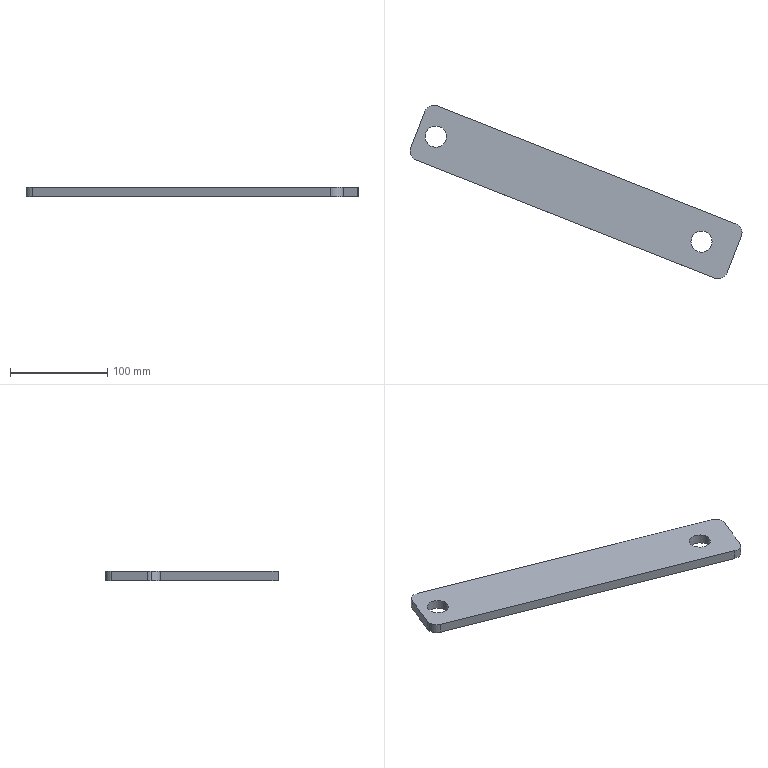Part | SolidWorks | features Extrusion 1 | 1 solid | 15 faces | box 341.614 x 178.454 x 10 mm | volume 201659 mm3 | cylinder 9 | plane 6 | commonest cylinder face diameters 20 x5 21.649 x2 22 x2
STEP:
#1=CARTESIAN_POINT('',(125.214,354.089,-1033.237));
#2=VERTEX_POINT('',#1);
#3=CARTESIAN_POINT('',(146.863,354.089,-1033.237));
#4=VERTEX_POINT('',#3);
#5=CARTESIAN_POINT('',(136.039,354.089,-1033.237));
#6=DIRECTION('',(0.,0.,1.));
#7=DIRECTION('',(1.,0.,0.));
#8=AXIS2_PLACEMENT_3D('',#5,#6,#7);
#9=CIRCLE('',#8,10.825);
#10=EDGE_CURVE('',#2,#4,#9,.T.);
#11=ORIENTED_EDGE('',*,*,#10,.T.);
#12=CARTESIAN_POINT('',(146.863,354.089,-1043.237));
#13=VERTEX_POINT('',#12);
#14=CARTESIAN_POINT('',(146.863,354.089,-1033.237));
#15=DIRECTION('',(0.,0.,-1.));
#16=VECTOR('',#15,1000.);
#17=LINE('',#14,#16);
#18=EDGE_CURVE('',#4,#13,#17,.T.);
#19=ORIENTED_EDGE('',*,*,#18,.T.);
#20=CARTESIAN_POINT('',(125.214,354.089,-1043.237));
#21=VERTEX_POINT('',#20);
#22=CARTESIAN_POINT('',(136.039,354.089,-1043.237));
#23=DIRECTION('',(0.,0.,1.));
#24=DIRECTION('',(1.,0.,0.));
#25=AXIS2_PLACEMENT_3D('',#22,#23,#24);
#26=CIRCLE('',#25,10.825);
#27=EDGE_CURVE('',#21,#13,#26,.T.);
#28=ORIENTED_EDGE('',*,*,#27,.F.);
#29=CARTESIAN_POINT('',(125.214,354.089,-1033.237));
#30=DIRECTION('',(0.,0.,-1.));
#31=VECTOR('',#30,1000.);
#32=LINE('',#29,#31);
#33=EDGE_CURVE('',#2,#21,#32,.T.);
#34=ORIENTED_EDGE('',*,*,#33,.F.);
#35=EDGE_LOOP('',(#11,#19,#28,#34));
#36=FACE_OUTER_BOUND('',#35,.T.);
#37=CARTESIAN_POINT('',(136.039,354.089,-1033.237));
#38=DIRECTION('',(0.,0.,-1.));
#39=DIRECTION('',(-1.,0.,0.));
#40=AXIS2_PLACEMENT_3D('',#37,#38,#39);
#41=CYLINDRICAL_SURFACE('',#40,10.825);
#42=ADVANCED_FACE('',(#36),#41,.F.);
#43=CARTESIAN_POINT('',(-148.238,462.051,-1033.237));
#44=VERTEX_POINT('',#43);
#45=CARTESIAN_POINT('',(-126.238,462.051,-1033.237));
#46=VERTEX_POINT('',#45);
#47=CARTESIAN_POINT('',(-137.238,462.051,-1033.237));
#48=DIRECTION('',(0.,0.,1.));
#49=DIRECTION('',(1.,0.,0.));
#50=AXIS2_PLACEMENT_3D('',#47,#48,#49);
#51=CIRCLE('',#50,11.);
#52=EDGE_CURVE('',#44,#46,#51,.T.);
#53=ORIENTED_EDGE('',*,*,#52,.T.);
#54=CARTESIAN_POINT('',(-126.238,462.051,-1043.237));
#55=VERTEX_POINT('',#54);
#56=CARTESIAN_POINT('',(-126.238,462.051,-1033.237));
#57=DIRECTION('',(0.,0.,-1.));
#58=VECTOR('',#57,1000.);
#59=LINE('',#56,#58);
#60=EDGE_CURVE('',#46,#55,#59,.T.);
#61=ORIENTED_EDGE('',*,*,#60,.T.);
#62=CARTESIAN_POINT('',(-148.238,462.051,-1043.237));
#63=VERTEX_POINT('',#62);
#64=CARTESIAN_POINT('',(-137.238,462.051,-1043.237));
#65=DIRECTION('',(0.,0.,1.));
#66=DIRECTION('',(1.,0.,0.));
#67=AXIS2_PLACEMENT_3D('',#64,#65,#66);
#68=CIRCLE('',#67,11.);
#69=EDGE_CURVE('',#63,#55,#68,.T.);
#70=ORIENTED_EDGE('',*,*,#69,.F.);
#71=CARTESIAN_POINT('',(-148.238,462.051,-1033.237));
#72=DIRECTION('',(0.,0.,-1.));
#73=VECTOR('',#72,1000.);
#74=LINE('',#71,#73);
#75=EDGE_CURVE('',#44,#63,#74,.T.);
#76=ORIENTED_EDGE('',*,*,#75,.F.);
#77=EDGE_LOOP('',(#53,#61,#70,#76));
#78=FACE_OUTER_BOUND('',#77,.T.);
#79=CARTESIAN_POINT('',(-137.238,462.051,-1033.237));
#80=DIRECTION('',(0.,0.,-1.));
#81=DIRECTION('',(-1.,0.,0.));
#82=AXIS2_PLACEMENT_3D('',#79,#80,#81);
#83=CYLINDRICAL_SURFACE('',#82,11.);
#84=ADVANCED_FACE('',(#78),#83,.F.);
#85=CARTESIAN_POINT('',(-163.887,447.124,-1033.237));
#86=VERTEX_POINT('',#85);
#87=CARTESIAN_POINT('',(-157.561,437.823,-1033.237));
#88=VERTEX_POINT('',#87);
#89=CARTESIAN_POINT('',(-153.887,447.124,-1033.237));
#90=DIRECTION('',(0.,0.,1.));
#91=DIRECTION('',(1.,0.,0.));
#92=AXIS2_PLACEMENT_3D('',#89,#90,#91);
#93=CIRCLE('',#92,10.);
#94=EDGE_CURVE('',#86,#88,#93,.T.);
#95=ORIENTED_EDGE('',*,*,#94,.F.);
#96=CARTESIAN_POINT('',(-163.887,447.124,-1043.237));
#97=VERTEX_POINT('',#96);
#98=CARTESIAN_POINT('',(-163.887,447.124,-1033.237));
#99=DIRECTION('',(0.,0.,-1.));
#100=VECTOR('',#99,1000.);
#101=LINE('',#98,#100);
#102=EDGE_CURVE('',#86,#97,#101,.T.);
#103=ORIENTED_EDGE('',*,*,#102,.T.);
#104=CARTESIAN_POINT('',(-157.561,437.823,-1043.237));
#105=VERTEX_POINT('',#104);
#106=CARTESIAN_POINT('',(-153.887,447.124,-1043.237));
#107=DIRECTION('',(0.,0.,1.));
#108=DIRECTION('',(1.,0.,0.));
#109=AXIS2_PLACEMENT_3D('',#106,#107,#108);
#110=CIRCLE('',#109,10.);
#111=EDGE_CURVE('',#97,#105,#110,.T.);
#112=ORIENTED_EDGE('',*,*,#111,.T.);
#113=CARTESIAN_POINT('',(-157.561,437.823,-1033.237));
#114=DIRECTION('',(0.,0.,-1.));
#115=VECTOR('',#114,1000.);
#116=LINE('',#113,#115);
#117=EDGE_CURVE('',#88,#105,#116,.T.);
#118=ORIENTED_EDGE('',*,*,#117,.F.);
#119=EDGE_LOOP('',(#95,#103,#112,#118));
#120=FACE_OUTER_BOUND('',#119,.T.);
#121=CARTESIAN_POINT('',(-153.887,447.124,-1033.237));
#122=DIRECTION('',(0.,0.,-1.));
#123=DIRECTION('',(-1.,0.,0.));
#124=AXIS2_PLACEMENT_3D('',#121,#122,#123);
#125=CYLINDRICAL_SURFACE('',#124,10.);
#126=ADVANCED_FACE('',(#120),#125,.T.);
#127=CARTESIAN_POINT('',(177.028,359.4,-1033.237));
#128=VERTEX_POINT('',#127);
#129=CARTESIAN_POINT('',(171.401,372.375,-1033.237));
#130=VERTEX_POINT('',#129);
#131=CARTESIAN_POINT('',(167.727,363.074,-1033.237));
#132=DIRECTION('',(0.,0.,1.));
#133=DIRECTION('',(-1.,0.,0.));
#134=AXIS2_PLACEMENT_3D('',#131,#132,#133);
#135=CIRCLE('',#134,10.);
#136=EDGE_CURVE('',#128,#130,#135,.T.);
#137=ORIENTED_EDGE('',*,*,#136,.T.);
#138=CARTESIAN_POINT('',(-135.516,493.626,-1033.237));
#139=VERTEX_POINT('',#138);
#140=CARTESIAN_POINT('',(-135.516,493.626,-1033.237));
#141=DIRECTION('',(-0.9301,0.3674,0.));
#142=VECTOR('',#141,1000.);
#143=LINE('',#140,#142);
#144=EDGE_CURVE('',#130,#139,#143,.T.);
#145=ORIENTED_EDGE('',*,*,#144,.T.);
#146=CARTESIAN_POINT('',(-148.491,488.,-1033.237));
#147=VERTEX_POINT('',#146);
#148=CARTESIAN_POINT('',(-139.19,484.326,-1033.237));
#149=DIRECTION('',(0.,0.,1.));
#150=DIRECTION('',(-1.,0.,0.));
#151=AXIS2_PLACEMENT_3D('',#148,#149,#150);
#152=CIRCLE('',#151,10.);
#153=EDGE_CURVE('',#139,#147,#152,.T.);
#154=ORIENTED_EDGE('',*,*,#153,.T.);
#155=CARTESIAN_POINT('',(-163.188,450.798,-1033.237));
#156=VERTEX_POINT('',#155);
#157=CARTESIAN_POINT('',(-148.491,488.,-1033.237));
#158=DIRECTION('',(-0.3674,-0.9301,0.));
#159=VECTOR('',#158,1000.);
#160=LINE('',#157,#159);
#161=EDGE_CURVE('',#147,#156,#160,.T.);
#162=ORIENTED_EDGE('',*,*,#161,.T.);
#163=CARTESIAN_POINT('',(-153.887,447.124,-1033.237));
#164=DIRECTION('',(0.,0.,1.));
#165=DIRECTION('',(1.,0.,0.));
#166=AXIS2_PLACEMENT_3D('',#163,#164,#165);
#167=CIRCLE('',#166,10.);
#168=EDGE_CURVE('',#156,#86,#167,.T.);
#169=ORIENTED_EDGE('',*,*,#168,.T.);
#170=ORIENTED_EDGE('',*,*,#94,.T.);
#171=CARTESIAN_POINT('',(149.356,316.572,-1033.237));
#172=VERTEX_POINT('',#171);
#173=CARTESIAN_POINT('',(-157.561,437.823,-1033.237));
#174=DIRECTION('',(0.9301,-0.3674,0.));
#175=VECTOR('',#174,1000.);
#176=LINE('',#173,#175);
#177=EDGE_CURVE('',#88,#172,#176,.T.);
#178=ORIENTED_EDGE('',*,*,#177,.T.);
#179=CARTESIAN_POINT('',(162.33,322.198,-1033.237));
#180=VERTEX_POINT('',#179);
#181=CARTESIAN_POINT('',(153.03,325.872,-1033.237));
#182=DIRECTION('',(0.,0.,1.));
#183=DIRECTION('',(-1.,0.,0.));
#184=AXIS2_PLACEMENT_3D('',#181,#182,#183);
#185=CIRCLE('',#184,10.);
#186=EDGE_CURVE('',#172,#180,#185,.T.);
#187=ORIENTED_EDGE('',*,*,#186,.T.);
#188=CARTESIAN_POINT('',(177.028,359.4,-1033.237));
#189=DIRECTION('',(0.3674,0.9301,0.));
#190=VECTOR('',#189,1000.);
#191=LINE('',#188,#190);
#192=EDGE_CURVE('',#180,#128,#191,.T.);
#193=ORIENTED_EDGE('',*,*,#192,.T.);
#194=EDGE_LOOP('',(#137,#145,#154,#162,#169,#170,#178,#187,#193));
#195=FACE_OUTER_BOUND('',#194,.T.);
#196=ORIENTED_EDGE('',*,*,#52,.F.);
#197=CARTESIAN_POINT('',(-137.238,462.051,-1033.237));
#198=DIRECTION('',(0.,0.,1.));
#199=DIRECTION('',(1.,0.,0.));
#200=AXIS2_PLACEMENT_3D('',#197,#198,#199);
#201=CIRCLE('',#200,11.);
#202=EDGE_CURVE('',#46,#44,#201,.T.);
#203=ORIENTED_EDGE('',*,*,#202,.F.);
#204=EDGE_LOOP('',(#196,#203));
#205=FACE_BOUND('',#204,.T.);
#206=ORIENTED_EDGE('',*,*,#10,.F.);
#207=CARTESIAN_POINT('',(136.039,354.089,-1033.237));
#208=DIRECTION('',(0.,0.,1.));
#209=DIRECTION('',(1.,0.,0.));
#210=AXIS2_PLACEMENT_3D('',#207,#208,#209);
#211=CIRCLE('',#210,10.825);
#212=EDGE_CURVE('',#4,#2,#211,.T.);
#213=ORIENTED_EDGE('',*,*,#212,.F.);
#214=EDGE_LOOP('',(#206,#213));
#215=FACE_BOUND('',#214,.T.);
#216=CARTESIAN_POINT('',(167.727,363.074,-1033.237));
#217=DIRECTION('',(0.,0.,-1.));
#218=DIRECTION('',(-1.,0.,0.));
#219=AXIS2_PLACEMENT_3D('',#216,#217,#218);
#220=PLANE('',#219);
#221=ADVANCED_FACE('',(#195,#205,#215),#220,.F.);
#222=ORIENTED_EDGE('',*,*,#69,.T.);
#223=CARTESIAN_POINT('',(-137.238,462.051,-1043.237));
#224=DIRECTION('',(0.,0.,1.));
#225=DIRECTION('',(1.,0.,0.));
#226=AXIS2_PLACEMENT_3D('',#223,#224,#225);
#227=CIRCLE('',#226,11.);
#228=EDGE_CURVE('',#55,#63,#227,.T.);
#229=ORIENTED_EDGE('',*,*,#228,.T.);
#230=EDGE_LOOP('',(#222,#229));
#231=FACE_BOUND('',#230,.T.);
#232=CARTESIAN_POINT('',(177.028,359.4,-1043.237));
#233=VERTEX_POINT('',#232);
#234=CARTESIAN_POINT('',(171.401,372.375,-1043.237));
#235=VERTEX_POINT('',#234);
#236=CARTESIAN_POINT('',(167.727,363.074,-1043.237));
#237=DIRECTION('',(0.,0.,1.));
#238=DIRECTION('',(-1.,0.,0.));
#239=AXIS2_PLACEMENT_3D('',#236,#237,#238);
#240=CIRCLE('',#239,10.);
#241=EDGE_CURVE('',#233,#235,#240,.T.);
#242=ORIENTED_EDGE('',*,*,#241,.F.);
#243=CARTESIAN_POINT('',(162.33,322.198,-1043.237));
#244=VERTEX_POINT('',#243);
#245=CARTESIAN_POINT('',(177.028,359.4,-1043.237));
#246=DIRECTION('',(0.3674,0.9301,0.));
#247=VECTOR('',#246,1000.);
#248=LINE('',#245,#247);
#249=EDGE_CURVE('',#244,#233,#248,.T.);
#250=ORIENTED_EDGE('',*,*,#249,.F.);
#251=CARTESIAN_POINT('',(149.356,316.572,-1043.237));
#252=VERTEX_POINT('',#251);
#253=CARTESIAN_POINT('',(153.03,325.872,-1043.237));
#254=DIRECTION('',(0.,0.,1.));
#255=DIRECTION('',(-1.,0.,0.));
#256=AXIS2_PLACEMENT_3D('',#253,#254,#255);
#257=CIRCLE('',#256,10.);
#258=EDGE_CURVE('',#252,#244,#257,.T.);
#259=ORIENTED_EDGE('',*,*,#258,.F.);
#260=CARTESIAN_POINT('',(-157.561,437.823,-1043.237));
#261=DIRECTION('',(0.9301,-0.3674,0.));
#262=VECTOR('',#261,1000.);
#263=LINE('',#260,#262);
#264=EDGE_CURVE('',#105,#252,#263,.T.);
#265=ORIENTED_EDGE('',*,*,#264,.F.);
#266=ORIENTED_EDGE('',*,*,#111,.F.);
#267=CARTESIAN_POINT('',(-163.188,450.798,-1043.237));
#268=VERTEX_POINT('',#267);
#269=CARTESIAN_POINT('',(-153.887,447.124,-1043.237));
#270=DIRECTION('',(0.,0.,1.));
#271=DIRECTION('',(1.,0.,0.));
#272=AXIS2_PLACEMENT_3D('',#269,#270,#271);
#273=CIRCLE('',#272,10.);
#274=EDGE_CURVE('',#268,#97,#273,.T.);
#275=ORIENTED_EDGE('',*,*,#274,.F.);
#276=CARTESIAN_POINT('',(-148.491,488.,-1043.237));
#277=VERTEX_POINT('',#276);
#278=CARTESIAN_POINT('',(-148.491,488.,-1043.237));
#279=DIRECTION('',(-0.3674,-0.9301,0.));
#280=VECTOR('',#279,1000.);
#281=LINE('',#278,#280);
#282=EDGE_CURVE('',#277,#268,#281,.T.);
#283=ORIENTED_EDGE('',*,*,#282,.F.);
#284=CARTESIAN_POINT('',(-135.516,493.626,-1043.237));
#285=VERTEX_POINT('',#284);
#286=CARTESIAN_POINT('',(-139.19,484.326,-1043.237));
#287=DIRECTION('',(0.,0.,1.));
#288=DIRECTION('',(-1.,0.,0.));
#289=AXIS2_PLACEMENT_3D('',#286,#287,#288);
#290=CIRCLE('',#289,10.);
#291=EDGE_CURVE('',#285,#277,#290,.T.);
#292=ORIENTED_EDGE('',*,*,#291,.F.);
#293=CARTESIAN_POINT('',(-135.516,493.626,-1043.237));
#294=DIRECTION('',(-0.9301,0.3674,0.));
#295=VECTOR('',#294,1000.);
#296=LINE('',#293,#295);
#297=EDGE_CURVE('',#235,#285,#296,.T.);
#298=ORIENTED_EDGE('',*,*,#297,.F.);
#299=EDGE_LOOP('',(#242,#250,#259,#265,#266,#275,#283,#292,#298));
#300=FACE_OUTER_BOUND('',#299,.T.);
#301=ORIENTED_EDGE('',*,*,#27,.T.);
#302=CARTESIAN_POINT('',(136.039,354.089,-1043.237));
#303=DIRECTION('',(0.,0.,1.));
#304=DIRECTION('',(1.,0.,0.));
#305=AXIS2_PLACEMENT_3D('',#302,#303,#304);
#306=CIRCLE('',#305,10.825);
#307=EDGE_CURVE('',#13,#21,#306,.T.);
#308=ORIENTED_EDGE('',*,*,#307,.T.);
#309=EDGE_LOOP('',(#301,#308));
#310=FACE_BOUND('',#309,.T.);
#311=CARTESIAN_POINT('',(167.727,363.074,-1043.237));
#312=DIRECTION('',(0.,0.,-1.));
#313=DIRECTION('',(-1.,0.,0.));
#314=AXIS2_PLACEMENT_3D('',#311,#312,#313);
#315=PLANE('',#314);
#316=ADVANCED_FACE('',(#231,#300,#310),#315,.T.);
#317=ORIENTED_EDGE('',*,*,#241,.T.);
#318=CARTESIAN_POINT('',(171.401,372.375,-1033.237));
#319=DIRECTION('',(0.,0.,-1.));
#320=VECTOR('',#319,1000.);
#321=LINE('',#318,#320);
#322=EDGE_CURVE('',#130,#235,#321,.T.);
#323=ORIENTED_EDGE('',*,*,#322,.F.);
#324=ORIENTED_EDGE('',*,*,#136,.F.);
#325=CARTESIAN_POINT('',(177.028,359.4,-1033.237));
#326=DIRECTION('',(0.,0.,-1.));
#327=VECTOR('',#326,1000.);
#328=LINE('',#325,#327);
#329=EDGE_CURVE('',#128,#233,#328,.T.);
#330=ORIENTED_EDGE('',*,*,#329,.T.);
#331=EDGE_LOOP('',(#317,#323,#324,#330));
#332=FACE_OUTER_BOUND('',#331,.T.);
#333=CARTESIAN_POINT('',(167.727,363.074,-1033.237));
#334=DIRECTION('',(0.,0.,-1.));
#335=DIRECTION('',(-1.,0.,0.));
#336=AXIS2_PLACEMENT_3D('',#333,#334,#335);
#337=CYLINDRICAL_SURFACE('',#336,10.);
#338=ADVANCED_FACE('',(#332),#337,.T.);
#339=ORIENTED_EDGE('',*,*,#297,.T.);
#340=CARTESIAN_POINT('',(-135.516,493.626,-1033.237));
#341=DIRECTION('',(0.,0.,-1.));
#342=VECTOR('',#341,1000.);
#343=LINE('',#340,#342);
#344=EDGE_CURVE('',#139,#285,#343,.T.);
#345=ORIENTED_EDGE('',*,*,#344,.F.);
#346=ORIENTED_EDGE('',*,*,#144,.F.);
#347=ORIENTED_EDGE('',*,*,#322,.T.);
#348=EDGE_LOOP('',(#339,#345,#346,#347));
#349=FACE_OUTER_BOUND('',#348,.T.);
#350=CARTESIAN_POINT('',(-135.516,493.626,-1033.237));
#351=DIRECTION('',(-0.3674,-0.9301,0.));
#352=DIRECTION('',(0.9301,-0.3674,0.));
#353=AXIS2_PLACEMENT_3D('',#350,#351,#352);
#354=PLANE('',#353);
#355=ADVANCED_FACE('',(#349),#354,.F.);
#356=ORIENTED_EDGE('',*,*,#291,.T.);
#357=CARTESIAN_POINT('',(-148.491,488.,-1033.237));
#358=DIRECTION('',(0.,0.,-1.));
#359=VECTOR('',#358,1000.);
#360=LINE('',#357,#359);
#361=EDGE_CURVE('',#147,#277,#360,.T.);
#362=ORIENTED_EDGE('',*,*,#361,.F.);
#363=ORIENTED_EDGE('',*,*,#153,.F.);
#364=ORIENTED_EDGE('',*,*,#344,.T.);
#365=EDGE_LOOP('',(#356,#362,#363,#364));
#366=FACE_OUTER_BOUND('',#365,.T.);
#367=CARTESIAN_POINT('',(-139.19,484.326,-1033.237));
#368=DIRECTION('',(0.,0.,-1.));
#369=DIRECTION('',(-1.,0.,0.));
#370=AXIS2_PLACEMENT_3D('',#367,#368,#369);
#371=CYLINDRICAL_SURFACE('',#370,10.);
#372=ADVANCED_FACE('',(#366),#371,.T.);
#373=ORIENTED_EDGE('',*,*,#282,.T.);
#374=CARTESIAN_POINT('',(-163.188,450.798,-1033.237));
#375=DIRECTION('',(0.,0.,-1.));
#376=VECTOR('',#375,1000.);
#377=LINE('',#374,#376);
#378=EDGE_CURVE('',#156,#268,#377,.T.);
#379=ORIENTED_EDGE('',*,*,#378,.F.);
#380=ORIENTED_EDGE('',*,*,#161,.F.);
#381=ORIENTED_EDGE('',*,*,#361,.T.);
#382=EDGE_LOOP('',(#373,#379,#380,#381));
#383=FACE_OUTER_BOUND('',#382,.T.);
#384=CARTESIAN_POINT('',(-148.491,488.,-1033.237));
#385=DIRECTION('',(0.9301,-0.3674,0.));
#386=DIRECTION('',(0.3674,0.9301,0.));
#387=AXIS2_PLACEMENT_3D('',#384,#385,#386);
#388=PLANE('',#387);
#389=ADVANCED_FACE('',(#383),#388,.F.);
#390=ORIENTED_EDGE('',*,*,#102,.F.);
#391=ORIENTED_EDGE('',*,*,#168,.F.);
#392=ORIENTED_EDGE('',*,*,#378,.T.);
#393=ORIENTED_EDGE('',*,*,#274,.T.);
#394=EDGE_LOOP('',(#390,#391,#392,#393));
#395=FACE_OUTER_BOUND('',#394,.T.);
#396=CARTESIAN_POINT('',(-153.887,447.124,-1033.237));
#397=DIRECTION('',(0.,0.,-1.));
#398=DIRECTION('',(-1.,0.,0.));
#399=AXIS2_PLACEMENT_3D('',#396,#397,#398);
#400=CYLINDRICAL_SURFACE('',#399,10.);
#401=ADVANCED_FACE('',(#395),#400,.T.);
#402=ORIENTED_EDGE('',*,*,#264,.T.);
#403=CARTESIAN_POINT('',(149.356,316.572,-1033.237));
#404=DIRECTION('',(0.,0.,-1.));
#405=VECTOR('',#404,1000.);
#406=LINE('',#403,#405);
#407=EDGE_CURVE('',#172,#252,#406,.T.);
#408=ORIENTED_EDGE('',*,*,#407,.F.);
#409=ORIENTED_EDGE('',*,*,#177,.F.);
#410=ORIENTED_EDGE('',*,*,#117,.T.);
#411=EDGE_LOOP('',(#402,#408,#409,#410));
#412=FACE_OUTER_BOUND('',#411,.T.);
#413=CARTESIAN_POINT('',(-157.561,437.823,-1033.237));
#414=DIRECTION('',(0.3674,0.9301,0.));
#415=DIRECTION('',(-0.9301,0.3674,0.));
#416=AXIS2_PLACEMENT_3D('',#413,#414,#415);
#417=PLANE('',#416);
#418=ADVANCED_FACE('',(#412),#417,.F.);
#419=ORIENTED_EDGE('',*,*,#258,.T.);
#420=CARTESIAN_POINT('',(162.33,322.198,-1033.237));
#421=DIRECTION('',(0.,0.,-1.));
#422=VECTOR('',#421,1000.);
#423=LINE('',#420,#422);
#424=EDGE_CURVE('',#180,#244,#423,.T.);
#425=ORIENTED_EDGE('',*,*,#424,.F.);
#426=ORIENTED_EDGE('',*,*,#186,.F.);
#427=ORIENTED_EDGE('',*,*,#407,.T.);
#428=EDGE_LOOP('',(#419,#425,#426,#427));
#429=FACE_OUTER_BOUND('',#428,.T.);
#430=CARTESIAN_POINT('',(153.03,325.872,-1033.237));
#431=DIRECTION('',(0.,0.,-1.));
#432=DIRECTION('',(-1.,0.,0.));
#433=AXIS2_PLACEMENT_3D('',#430,#431,#432);
#434=CYLINDRICAL_SURFACE('',#433,10.);
#435=ADVANCED_FACE('',(#429),#434,.T.);
#436=ORIENTED_EDGE('',*,*,#249,.T.);
#437=ORIENTED_EDGE('',*,*,#329,.F.);
#438=ORIENTED_EDGE('',*,*,#192,.F.);
#439=ORIENTED_EDGE('',*,*,#424,.T.);
#440=EDGE_LOOP('',(#436,#437,#438,#439));
#441=FACE_OUTER_BOUND('',#440,.T.);
#442=CARTESIAN_POINT('',(177.028,359.4,-1033.237));
#443=DIRECTION('',(-0.9301,0.3674,0.));
#444=DIRECTION('',(-0.3674,-0.9301,0.));
#445=AXIS2_PLACEMENT_3D('',#442,#443,#444);
#446=PLANE('',#445);
#447=ADVANCED_FACE('',(#441),#446,.F.);
#448=ORIENTED_EDGE('',*,*,#60,.F.);
#449=ORIENTED_EDGE('',*,*,#202,.T.);
#450=ORIENTED_EDGE('',*,*,#75,.T.);
#451=ORIENTED_EDGE('',*,*,#228,.F.);
#452=EDGE_LOOP('',(#448,#449,#450,#451));
#453=FACE_OUTER_BOUND('',#452,.T.);
#454=CARTESIAN_POINT('',(-137.238,462.051,-1033.237));
#455=DIRECTION('',(0.,0.,-1.));
#456=DIRECTION('',(-1.,0.,0.));
#457=AXIS2_PLACEMENT_3D('',#454,#455,#456);
#458=CYLINDRICAL_SURFACE('',#457,11.);
#459=ADVANCED_FACE('',(#453),#458,.F.);
#460=ORIENTED_EDGE('',*,*,#18,.F.);
#461=ORIENTED_EDGE('',*,*,#212,.T.);
#462=ORIENTED_EDGE('',*,*,#33,.T.);
#463=ORIENTED_EDGE('',*,*,#307,.F.);
#464=EDGE_LOOP('',(#460,#461,#462,#463));
#465=FACE_OUTER_BOUND('',#464,.T.);
#466=CARTESIAN_POINT('',(136.039,354.089,-1033.237));
#467=DIRECTION('',(0.,0.,-1.));
#468=DIRECTION('',(-1.,0.,0.));
#469=AXIS2_PLACEMENT_3D('',#466,#467,#468);
#470=CYLINDRICAL_SURFACE('',#469,10.825);
#471=ADVANCED_FACE('',(#465),#470,.F.);
#472=CLOSED_SHELL('',(#42,#84,#126,#221,#316,#338,#355,#372,#389,#401,#418,#435,#447,#459,#471));
#473=MANIFOLD_SOLID_BREP('',#472);
#474=CARTESIAN_POINT('',(0.,0.,0.));
#475=DIRECTION('',(0.,0.,1.));
#476=DIRECTION('',(1.,0.,0.));
#477=AXIS2_PLACEMENT_3D('',#474,#475,#476);
#478=(LENGTH_UNIT()NAMED_UNIT(*)SI_UNIT(.MILLI.,.METRE.));
#479=UNCERTAINTY_MEASURE_WITH_UNIT(LENGTH_MEASURE(0.00001),#478,'','');
#480=(NAMED_UNIT(*)PLANE_ANGLE_UNIT()SI_UNIT($,.RADIAN.));
#481=(NAMED_UNIT(*)SI_UNIT($,.STERADIAN.)SOLID_ANGLE_UNIT());
#482=(GEOMETRIC_REPRESENTATION_CONTEXT(3)GLOBAL_UNCERTAINTY_ASSIGNED_CONTEXT((#479))GLOBAL_UNIT_ASSIGNED_CONTEXT((#478,#480,#481))REPRESENTATION_CONTEXT('',''));
#483=ADVANCED_BREP_SHAPE_REPRESENTATION('',(#473,#477),#482);